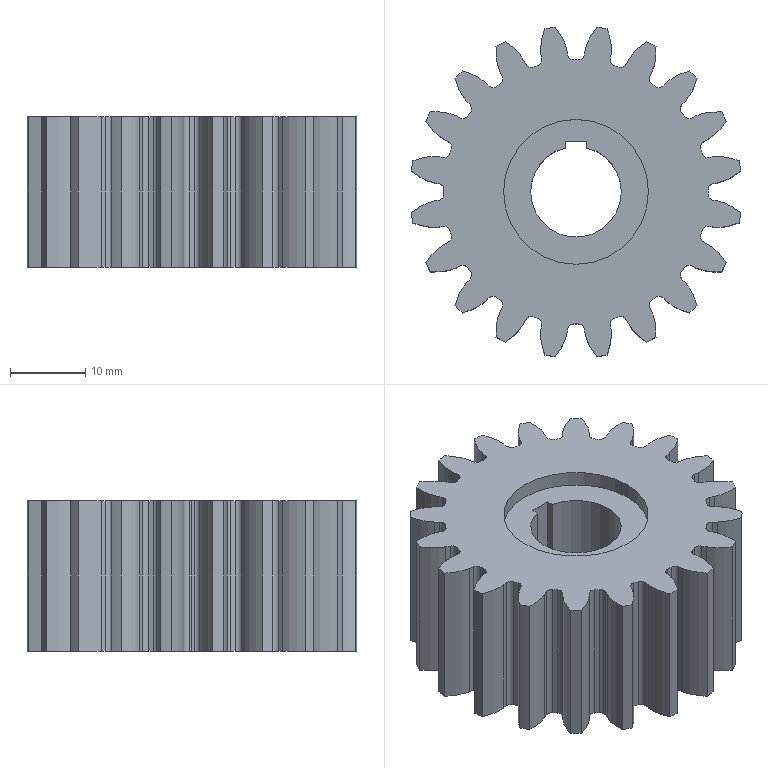Part | SolidWorks | features ICE 4, Extrusion 1 | 1 solid | 185 faces | box 43.654 x 43.654 x 20 mm | volume 21667 mm3 | cylinder 98 | plane 47 | spline 40 | commonest cylinder face diameters 1.52 x50 35 x21 44 x20 19.2 x4 12 x3